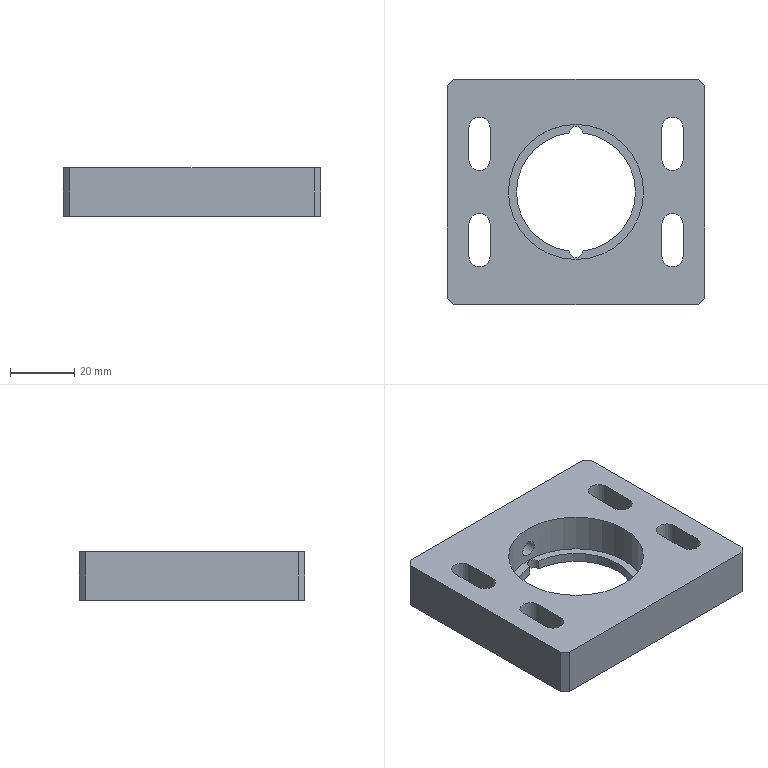CAM job | NX | 3-axis milling, drilling | part box 80 x 70 x 15 mm | stock box 80 x 70 x 15 mm
Tools:
number,name,description,diameter,corner_radius,flute_length,length,flutes
4,D4,平底铣刀-粗,4.0,0.0,25.0,75.0,2
6,D6,平底铣刀-粗,6.0,0.0,25.0,75.0,2
9,D10,平底铣刀-粗,10.0,0.0,35.0,75.0,2
11,D3-J,平底铣刀-精,3.0,0.0,50.0,75.0,2
7,D6-J,平底铣刀-精,6.0,0.0,25.0,75.0,2
10,D10-J,平底铣刀-精,10.0,0.0,35.0,75.0,2
2,D6倒角刀,倒角刀,6.0,0.0,3.0,25.0,2
20,M3X0.5,丝锥,2.5,0.0,35.0,50.0,2
1,C6定点钻,倒角刀,6.0,0.0,3.0,3.0,2
12,ZT2.6,钻头,2.6,0.0,35.0,50.0,2
Operations:
program,operation,operation_type,tool,method,geometry_group,spindle_rpm,surface_speed,feed_per_tooth,feed_cut,feed_plunge,cut_length_mm,path_length_mm,cut_time_min,machine_time_min
B,选线往复层切开粗-中_COPY_1,PlanarMilling,D10,分层开粗-切深K-步距G,W-B,3000.0,94.245,0.3333,2000.0,100.0,1333.019,2035.977,0.6665,0.7368
B,型腔铣开粗-中_COPY_1,CavityMilling,D10,分层开粗-切深K-步距G,W-B,3000.0,94.245,0.3333,2000.0,100.0,5671.538,6087.707,2.836,2.897
B,平面去毛刺6X45L_COPY_1,SurfaceContour,D6倒角刀,爬面_倒角-切深0-步距G,W-B,3500.0,65.972,0.1429,1000.0,100.0,739.249,1162.801,0.7392,0.7816
B,平面铣精光侧面-中-直线_COPY_1,PlanarMilling,D10-J,侧刃精光-切深K-步距G,W-B,3000.0,94.245,0.1333,800.0,100.0,67.314,727.071,0.0841,0.1501
B,底壁铣精光侧面-中_COPY,VolumeBased25DMillingOperation,D10-J,侧刃精光-切深K-步距G,W-B,3000.0,94.248,0.1333,800.0,100.0,218.649,260.523,0.2733,0.2775
B,底壁铣精光侧面-中_COPY_COPY,VolumeBased25DMillingOperation,D10-J,侧刃精光-切深K-步距G,W-B,3000.0,94.248,0.1333,800.0,100.0,218.649,260.523,0.2733,0.2775
A,选线往复层切开粗-中_COPY,PlanarMilling,D10,分层开粗-切深K-步距G,W-A,3000.0,94.245,0.3333,2000.0,100.0,1333.019,2035.977,0.6665,0.7368
A,型腔铣开粗-中_COPY,CavityMilling,D10,分层开粗-切深K-步距G,W-A,3000.0,94.245,0.3333,2000.0,100.0,1622.417,1760.824,0.8112,0.8308
A,打点-深0.8,Operation,C6定点钻,NONE,W-A,3000.0,56.0,0.01,60.0,90.0,7.2,218.659,0.12,0.1411
A,盲锥孔-M3螺纹底孔,Operation,ZT2.6,NONE,W-A,2000.0,15.708,0.0125,50.0,90.0,40.0,284.259,0.8,0.8244
A,盲腰槽粗,VolumeBased25DMillingOperation,D6,METHOD,W-A,3500.0,65.973,0.1714,1200.0,100.0,4075.336,4626.555,3.396,3.451
A,通腰槽粗_1,VolumeBased25DMillingOperation,D4,METHOD,W-A,3000.0,37.699,0.2,1200.0,100.0,6835.975,7438.977,5.697,5.757
A,腰槽精,VolumeBased25DMillingOperation,D6-J,METHOD,W-A,3200.0,32.0,0.1143,600.0,100.0,303.49,915.238,0.5058,0.567
A,清角D4,ZLevelMilling,D3-J,METHOD,W-A,3500.0,75.0,0.25,1500.0,80.0,296.534,533.755,0.1982,0.222
A,腰槽精_3,VolumeBased25DMillingOperation,D3-J,METHOD,W-A,3200.0,32.0,0.0781,500.0,100.0,268.304,951.206,0.5366,0.6049
A,框半精_1,VolumeBased25DMillingOperation,D6-J,METHOD,W-A,3200.0,157.0,0.2,800.0,90.0,103.077,209.077,0.1291,0.1397
A,框精_1,VolumeBased25DMillingOperation,D6-J,METHOD,W-A,3200.0,157.0,0.2,800.0,90.0,102.877,208.877,0.1289,0.1395
A,钻倒角_1,Operation,D6倒角刀,METHOD,W-A,4000.0,75.398,0.01,80.0,0.0,19.0,248.729,0.2375,0.2605
A,平面去毛刺6X45L_COPY,SurfaceContour,D6倒角刀,爬面_倒角-切深0-步距G,W-A,3500.0,65.972,0.1429,1000.0,100.0,631.574,1010.342,0.6316,0.6695
A,盲锥孔-攻牙M3,Operation,M3X0.5,METHOD,W-A,800.0,6.283,0.0003,0.5,90.0,26.0,256.259,52.0,52.023
A,平面铣精光侧面-中-直线_COPY,PlanarMilling,D10-J,侧刃精光-切深K-步距G,W-A,3000.0,94.245,0.1333,800.0,100.0,67.314,727.071,0.0841,0.1501